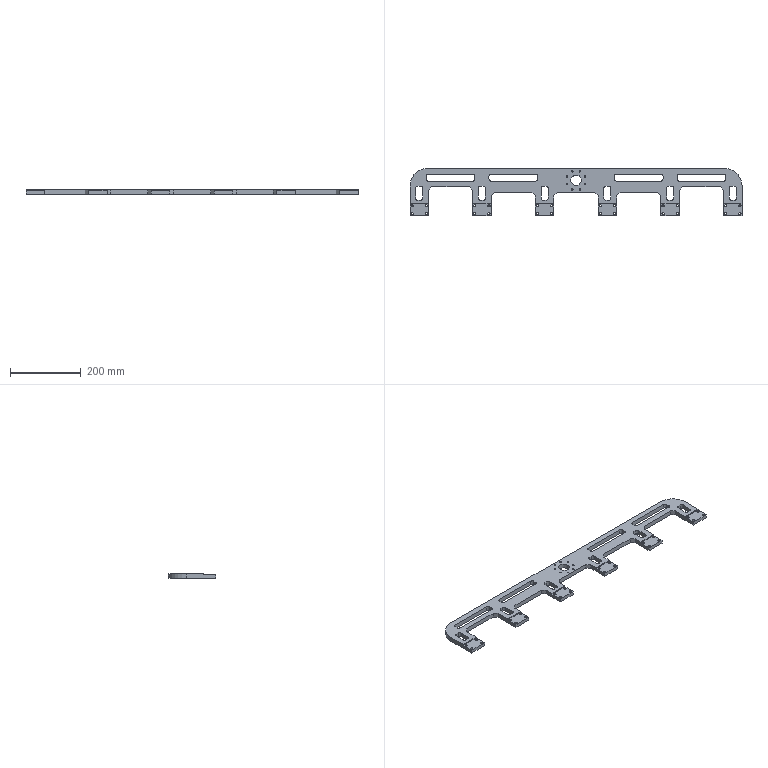NC program | NX | posted with a generic post | part box 941 x 134 x 13 mm
Lines 3851 to 4152 of 4152:
(PLANAR_MILL_COPY_1_COPY , TOOL : D6A45)
N7652 T07 M6
N7654 G54
N7656 G17 G0 G90 X81. Y-2.13 S9500 M3
N7658 G43 Z30. H7
N7660 Z0.
N7662 G94 G1 Z-1. F1400.
N7664 X80.3 Y-2.534
N7666 G3 X79.8 Y-3.4 R1.
N7668 G1 Y-17.4
N7670 G3 X84.9 Y-22.5 R5.1
N7672 G1 X92.9
N7674 G3 X98. Y-17.4 R5.1
N7676 G1 Y10.6
N7678 G3 X92.9 Y15.7 R5.1
N7680 G1 X84.9
N7682 G3 X79.8 Y10.6 R5.1
N7684 G1 Y-3.4
N7686 G3 X80.3 Y-4.266 R1.
N7688 G1 X81. Y-4.67
N7690 Z0.
N7692 G0 Z30.
N7694 X179.07 Y48.9
N7696 Z0.
N7698 G1 Z-1.
N7700 X178.666 Y49.6
N7702 G3 X177.8 Y50.1 R1.
N7704 G1 X114.9
N7706 G3 X109.8 Y45. R5.1
N7708 G1 Y37.
N7710 G3 X114.9 Y31.9 R5.1
N7712 G1 X240.7
N7714 G3 X245.8 Y37. R5.1
N7716 G1 Y45.
N7718 G3 X240.7 Y50.1 R5.1
N7720 G1 X177.8
N7722 G3 X176.934 Y49.6 R1.
N7724 G1 X176.53 Y48.9
N7726 Z0.
N7728 G0 Z30.
N7730 X258.8 Y-2.13
N7732 Z0.
N7734 G1 Z-1.
N7736 X258.1 Y-2.534
N7738 G3 X257.6 Y-3.4 R1.
N7740 G1 Y-17.4
N7742 G3 X262.7 Y-22.5 R5.1
N7744 G1 X270.7
N7746 G3 X275.8 Y-17.4 R5.1
N7748 G1 Y10.6
N7750 G3 X270.7 Y15.7 R5.1
N7752 G1 X262.7
N7754 G3 X257.6 Y10.6 R5.1
N7756 G1 Y-3.4
N7758 G3 X258.1 Y-4.266 R1.
N7760 G1 X258.8 Y-4.67
N7762 Z0.
N7764 G0 Z30.
N7766 X51.819 Y69.1
N7768 Z0.
N7770 G1 Z-1.
N7772 X52.223 Y68.4
N7774 G3 X53.089 Y67.9 R1.
N7776 G1 X420.5
N7778 G2 X471.4 Y17. R50.9
N7780 G1 Y-33.3
N7782 G2 X470.4 Y-34.3 R1.
N7784 G1 X418.6
N7786 G2 X417.6 Y-33.3 R1.
N7788 G1 Y4.627
N7790 X408.127 Y14.1
N7792 X303.073
N7794 X293.6 Y4.627
N7796 Y-33.3
N7798 G2 X292.6 Y-34.3 R1.
N7800 G1 X240.8
N7802 G2 X239.8 Y-33.3 R1.
N7804 G1 Y-11.328
N7806 X230.327 Y-1.855
N7808 X125.273
N7810 X115.8 Y-11.328
N7812 Y-33.3
N7814 G2 X114.8 Y-34.3 R1.
N7816 G1 X63.
N7818 G2 X62. Y-33.3 R1.
N7820 G1 Y-11.328
N7822 X53.089 Y-2.417
N7824 G3 X52.123 Y-2.158 R1.
N7826 G1 X52.03 Y-3.055
N7828 Z0.
N7830 G0 Z30.
N7832 X356.87 Y48.9
N7834 Z0.
N7836 G1 Z-1.
N7838 X356.466 Y49.6
N7840 G3 X355.6 Y50.1 R1.
N7842 G1 X292.7
N7844 G3 X287.6 Y45. R5.1
N7846 G1 Y37.
N7848 G3 X292.7 Y31.9 R5.1
N7850 G1 X418.5
N7852 G3 X423.6 Y37. R5.1
N7854 G1 Y45.
N7856 G3 X418.5 Y50.1 R5.1
N7858 G1 X355.6
N7860 G3 X354.734 Y49.6 R1.
N7862 G1 X354.33 Y48.9
N7864 Z0.
N7866 G0 Z30.
N7868 X452.4 Y-4.67
N7870 Z0.
N7872 G1 Z-1.
N7874 X453.1 Y-4.266
N7876 G3 X453.6 Y-3.4 R1.
N7878 G1 Y10.6
N7880 G3 X448.5 Y15.7 R5.1
N7882 G1 X440.5
N7884 G3 X435.4 Y10.6 R5.1
N7886 G1 Y-17.4
N7888 G3 X440.5 Y-22.5 R5.1
N7890 G1 X448.5
N7892 G3 X453.6 Y-17.4 R5.1
N7894 G1 Y-3.4
N7896 G3 X453.1 Y-2.534 R1.
N7898 G1 X452.4 Y-2.13
N7900 Z0.
N7902 G0 Z30.
(PLANAR_MILL_COPY_COPY_COPY , TOOL : D6A45)
N7904 X68.893 Y-38.1
N7906 Z-3.
N7908 G1 Z-4.
N7910 Y-37.056
N7912 G3 X68.418 Y-36.9 R0.5
N7914 X69.382 Y-36.9 R-2.35
N7916 X68.907 Y-37.056 R0.5
N7918 G1 Y-38.1
N7920 Z-3.
N7922 G0 Z30.
N7924 X68.412 Y-62.242
N7926 Z-3.
N7928 G1 Z-4.
N7930 X68.034 Y-63.05
N7932 G3 X68.9 Y-63.55 R1.
N7934 X71.25 Y-61.2 R2.35
N7936 X68.9 Y-63.55 R-2.35
N7938 X69.766 Y-63.05 R1.
N7940 G1 X69.388 Y-62.242
N7942 Z-3.
N7944 G0 Z30.
N7946 X117.213 Y-37.492
N7948 Z-3.
N7950 G1 Z-4.
N7952 X116.765 Y-37.043
N7954 G3 X115.8 Y-36.782 R1.
N7956 G1 Y-66.9
N7958 G2 X114.8 Y-67.9 R1.
N7960 G1 X63.
N7962 G2 X62. Y-66.9 R1.
N7964 G1 Y-36.782
N7966 G3 X61.035 Y-37.043 R1.
N7968 G1 X60.587 Y-37.492
N7970 Z-3.
N7972 G0 Z30.
N7974 X472.813
N7976 Z-3.
N7978 G1 Z-4.
N7980 X472.365 Y-37.043
N7982 G3 X471.4 Y-36.782 R1.
N7984 G1 Y-66.9
N7986 G2 X470.4 Y-67.9 R1.
N7988 G1 X418.6
N7990 G2 X417.6 Y-66.9 R1.
N7992 G1 Y-36.782
N7994 G3 X416.635 Y-37.043 R1.
N7996 G1 X416.187 Y-37.492
N7998 Z-3.
N8000 G0 Z30.
N8002 X295.013
N8004 Z-3.
N8006 G1 Z-4.
N8008 X294.565 Y-37.043
N8010 G3 X293.6 Y-36.782 R1.
N8012 G1 Y-66.9
N8014 G2 X292.6 Y-67.9 R1.
N8016 G1 X240.8
N8018 G2 X239.8 Y-66.9 R1.
N8020 G1 Y-36.782
N8022 G3 X238.835 Y-37.043 R1.
N8024 G1 X238.387 Y-37.492
N8026 Z-3.
N8028 G0 Z30.
N8030 X108.412 Y-62.242
N8032 Z-3.
N8034 G1 Z-4.
N8036 X108.034 Y-63.05
N8038 G3 X108.9 Y-63.55 R1.
N8040 X111.25 Y-61.2 R2.35
N8042 X108.9 Y-63.55 R-2.35
N8044 X109.766 Y-63.05 R1.
N8046 G1 X109.388 Y-62.242
N8048 Z-3.
N8050 G0 Z30.
N8052 X108.893 Y-38.1
N8054 Z-3.
N8056 G1 Z-4.
N8058 Y-37.056
N8060 G3 X108.418 Y-36.9 R0.5
N8062 X109.382 Y-36.9 R-2.35
N8064 X108.907 Y-37.056 R0.5
N8066 G1 Y-38.1
N8068 Z-3.
N8070 G0 Z30.
N8072 X246.693
N8074 Z-3.
N8076 G1 Z-4.
N8078 Y-37.056
N8080 G3 X246.218 Y-36.9 R0.5
N8082 X247.182 Y-36.9 R-2.35
N8084 X246.707 Y-37.056 R0.5
N8086 G1 Y-38.1
N8088 Z-3.
N8090 G0 Z30.
N8092 X246.212 Y-62.242
N8094 Z-3.
N8096 G1 Z-4.
N8098 X245.834 Y-63.05
N8100 G3 X246.7 Y-63.55 R1.
N8102 X249.05 Y-61.2 R2.35
N8104 X246.7 Y-63.55 R-2.35
N8106 X247.566 Y-63.05 R1.
N8108 G1 X247.188 Y-62.242
N8110 Z-3.
N8112 G0 Z30.
N8114 X286.212
N8116 Z-3.
N8118 G1 Z-4.
N8120 X285.834 Y-63.05
N8122 G3 X286.7 Y-63.55 R1.
N8124 X289.05 Y-61.2 R2.35
N8126 X286.7 Y-63.55 R-2.35
N8128 X287.566 Y-63.05 R1.
N8130 G1 X287.188 Y-62.242
N8132 Z-3.
N8134 G0 Z30.
N8136 X286.693 Y-38.1
N8138 Z-3.
N8140 G1 Z-4.
N8142 Y-37.056
N8144 G3 X286.218 Y-36.9 R0.5
N8146 X287.182 Y-36.9 R-2.35
N8148 X286.707 Y-37.056 R0.5
N8150 G1 Y-38.1
N8152 Z-3.
N8154 G0 Z30.
N8156 X424.493
N8158 Z-3.
N8160 G1 Z-4.
N8162 Y-37.056
N8164 G3 X424.018 Y-36.9 R0.5
N8166 X424.982 Y-36.9 R-2.35
N8168 X424.507 Y-37.056 R0.5
N8170 G1 Y-38.1
N8172 Z-3.
N8174 G0 Z30.
N8176 X424.012 Y-62.242
N8178 Z-3.
N8180 G1 Z-4.
N8182 X423.634 Y-63.05
N8184 G3 X424.5 Y-63.55 R1.
N8186 X426.85 Y-61.2 R2.35
N8188 X424.5 Y-63.55 R-2.35
N8190 X425.366 Y-63.05 R1.
N8192 G1 X424.988 Y-62.242
N8194 Z-3.
N8196 G0 Z30.
N8198 X464.012
N8200 Z-3.
N8202 G1 Z-4.
N8204 X463.634 Y-63.05
N8206 G3 X464.5 Y-63.55 R1.
N8208 X466.85 Y-61.2 R2.35
N8210 X464.5 Y-63.55 R-2.35
N8212 X465.366 Y-63.05 R1.
N8214 G1 X464.988 Y-62.242
N8216 Z-3.
N8218 G0 Z30.
N8220 X464.493 Y-38.1
N8222 Z-3.
N8224 G1 Z-4.
N8226 Y-37.056
N8228 G3 X464.018 Y-36.9 R0.5
N8230 X464.982 Y-36.9 R-2.35
N8232 X464.507 Y-37.056 R0.5
N8234 G1 Y-38.1
N8236 Z-3.
N8238 G0 Z30.
N8240 M5
N8242 M2